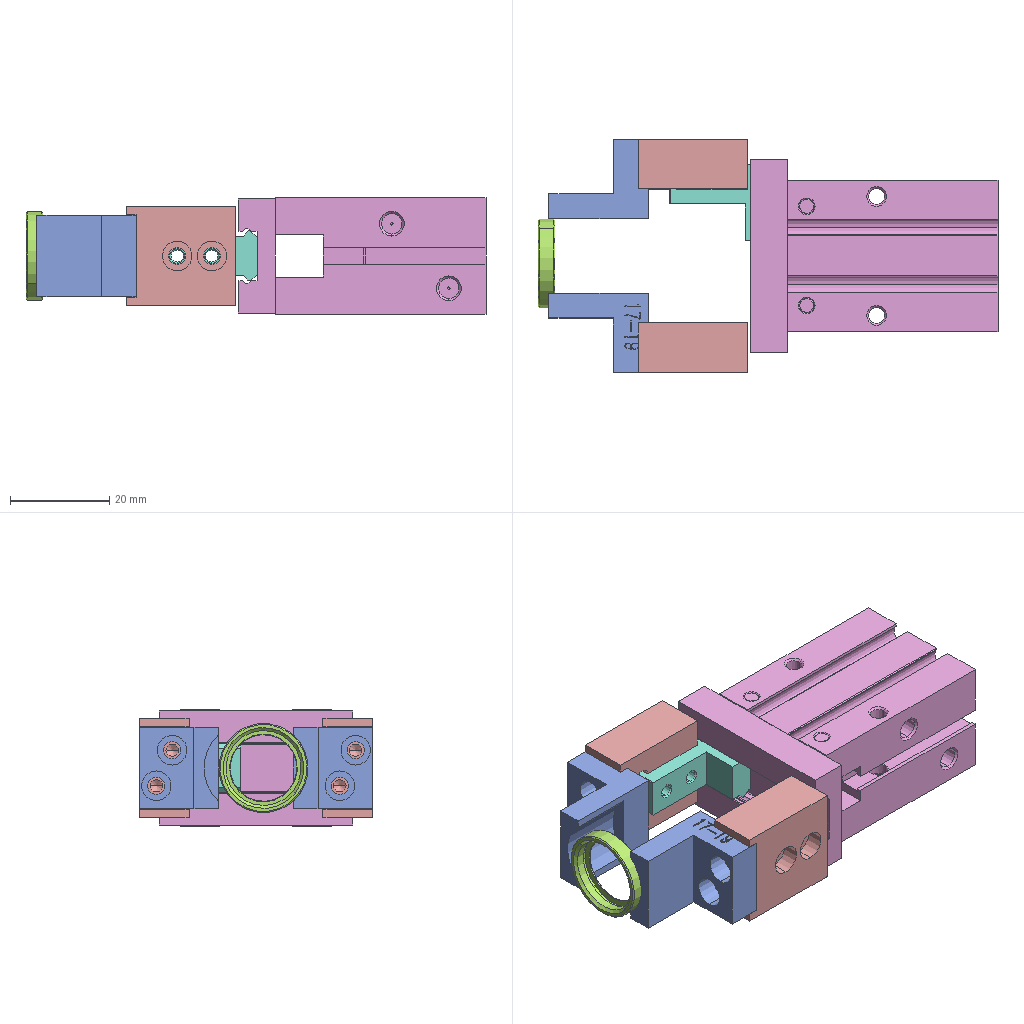Assembly | SolidWorks | 7 different items | 9 placed | box 93 x 47 x 24 mm
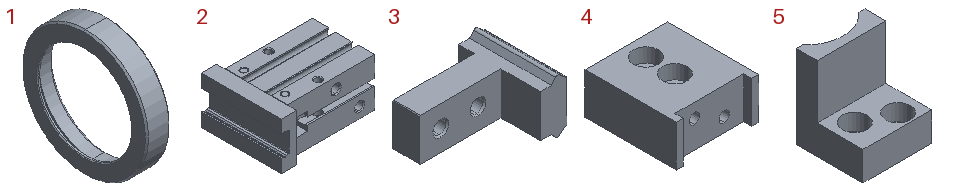Parts list (item | name | quantity | size | volume | features):
1 | - | x1 | 3.414 x 18 x 18 mm | 239.463 mm3 | features Revolution 1
2 | - | x1 | 50 x 39 x 23.5 mm | 27612 mm3 | features BaseBody 1
3 | - | x1 | 20.3 x 15.4 x 10.1 mm | 1229 mm3 | features BaseBody 1
4 | - | x2 | 20 x 22 x 10 mm | 3468 mm3 | features MBimport 1
5 | - | x2 | 16.5 x 16 x 20 mm | 2274 mm3 | features ICE 3, Extrusion 1, HoleWzd 1
6 | HFZ16((CL)) | x1 | - | - | -
7 | HFZ16(CL)_fl | x1 | - | - | -
Mates (type | each side: item.copy, entity, surface, feature):
Coincident | 3.1 face plane HFZ16(CL)_fr | 2.1 face plane HFZ16(CL)_body
Width | 2.1 face plane HFZ16(CL)_body | 2.1 face plane HFZ16(CL)_body | 3.1 face plane HFZ16(CL)_fr | 3.1 face plane HFZ16(CL)_fr
Concentric | 4.1 face cylinder PN_0001 short gripper arm seat.STEP | 3.1 face cylinder HFZ16(CL)_fr | 2 times
Coincident | 4.1 face plane PN_0001 short gripper arm seat.STEP | 3.1 face plane HFZ16(CL)_fr
Coincident | 4.2 face plane PN_0001 short gripper arm seat.STEP | 5.1 face plane Boss-Extrude1
Concentric | 4.2 face cylinder PN_0001 short gripper arm seat.STEP | 5.1 face cylinder CBORE for M3 Hex Head Bolt1 | 5 times
Coincident | 4.1 face plane PN_0001 short gripper arm seat.STEP | 5.2 face plane Boss-Extrude1
Concentric | 4.1 face cylinder PN_0001 short gripper arm seat.STEP | 5.2 face cylinder CBORE for M3 Hex Head Bolt1 | 2 times
Concentric | 5.1 face cylinder Cut-Extrude2 | 1.1 face cylinder Revolve1